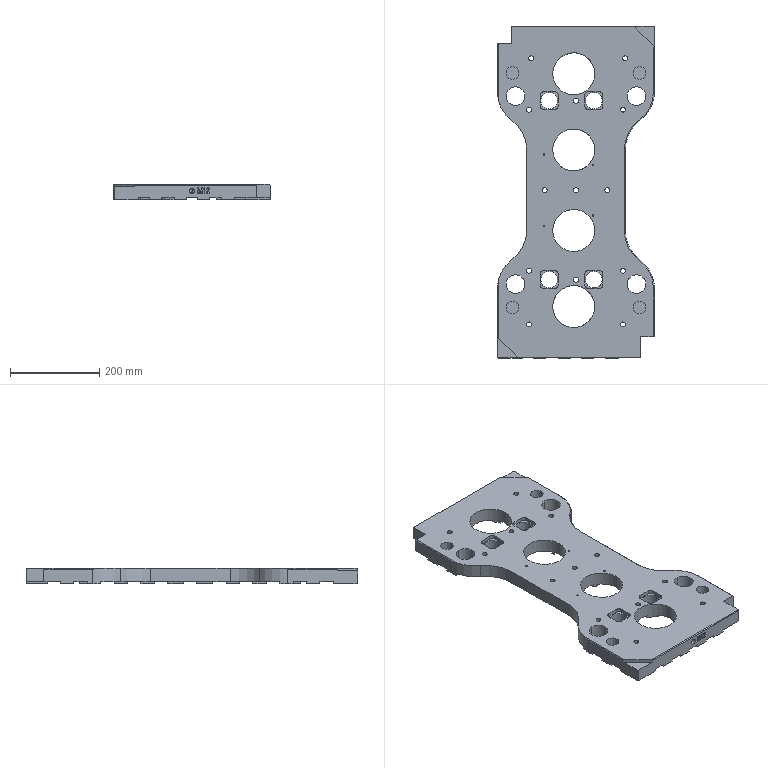Part | Creo | 1 solid | 623 faces | box 350 x 742 x 35 mm | volume 5530348 mm3 | plane 392 | cylinder 129 | other 94 | cone 8 | commonest cylinder face diameters 11 x26 18 x26 16 x16 3.8 x8 28 x8 37 x8